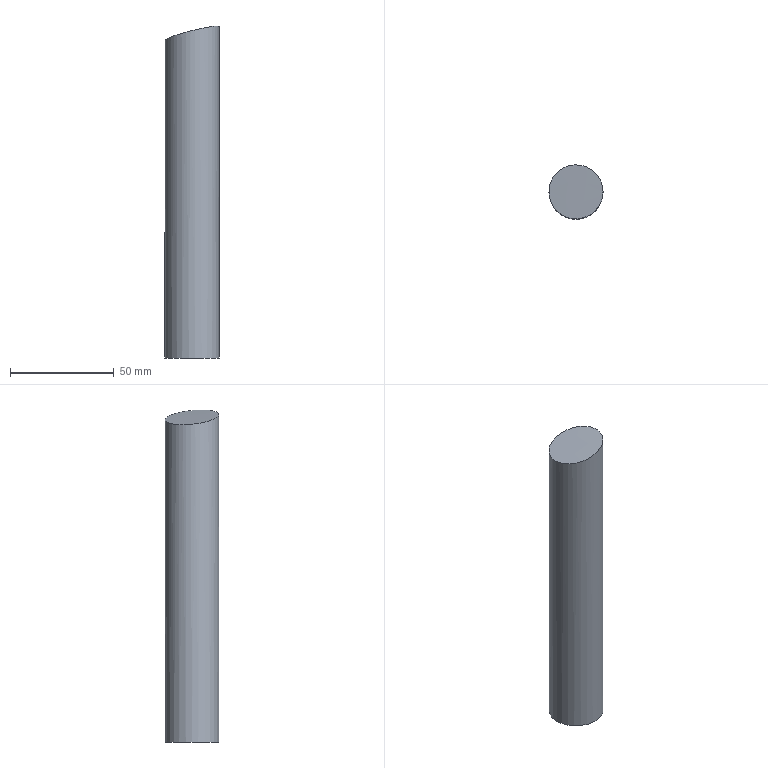Part | NX | features solid 2 | 1 solid | 3 faces | box 26 x 26 x 159.758 mm | volume 82970 mm3 | cylinder 1 | plane 1 | spline 1 | commonest cylinder face diameters 26 x1
STEP:
#1=CARTESIAN_POINT('',(-792.,330.,-138.));
#2=VERTEX_POINT('',#1);
#3=CARTESIAN_POINT('',(-805.,330.,-138.));
#4=DIRECTION('',(0.,0.,-1.));
#5=DIRECTION('',(1.,0.,0.));
#6=AXIS2_PLACEMENT_3D('',#3,#4,#5);
#7=CIRCLE('',#6,13.);
#8=EDGE_CURVE('',#2,#2,#7,.T.);
#9=ORIENTED_EDGE('',*,*,#8,.F.);
#10=EDGE_LOOP('',(#9));
#11=FACE_BOUND('',#10,.T.);
#12=CARTESIAN_POINT('',(-802.129,342.679,17.767));
#13=VERTEX_POINT('',#12);
#14=CARTESIAN_POINT('',(-794.433,338.853,20.068));
#15=CARTESIAN_POINT('',(-801.821,343.999,17.725));
#16=CARTESIAN_POINT('',(-810.751,342.544,15.59));
#17=CARTESIAN_POINT('',(-815.875,337.741,14.744));
#18=CARTESIAN_POINT('',(-818.033,332.897,14.664));
#19=CARTESIAN_POINT('',(-818.129,327.615,15.161));
#20=CARTESIAN_POINT('',(-815.561,321.141,16.463));
#21=CARTESIAN_POINT('',(-808.205,316.014,18.844));
#22=CARTESIAN_POINT('',(-799.271,317.444,20.936));
#23=CARTESIAN_POINT('',(-794.136,322.243,21.743));
#24=CARTESIAN_POINT('',(-791.968,327.089,21.811));
#25=CARTESIAN_POINT('',(-791.871,332.386,21.326));
#26=CARTESIAN_POINT('',(-794.433,338.853,20.068));
#27=CARTESIAN_POINT('',(-801.821,343.999,17.725));
#28=CARTESIAN_POINT('',(-810.751,342.544,15.59));
#29=B_SPLINE_CURVE_WITH_KNOTS('',3,(#14,#15,#16,#17,#18,#19,#20,#21,#22,#23,#24,#25,#26,#27,#28),.UNSPECIFIED.,.T.,.F.,(1,1,1,1,1,1,1,1,1,1,1,1,1,1,1,1,1,1,1),(-0.02068,-0.01551,-0.01034,0.,0.01034,0.01551,0.02068,0.02585,0.03102,0.04136,0.0517,0.05687,0.06204,0.06721,0.07238,0.08272,0.09306,0.09823,0.1034),.UNSPECIFIED.);
#30=EDGE_CURVE('',#13,#13,#29,.T.);
#31=ORIENTED_EDGE('',*,*,#30,.F.);
#32=EDGE_LOOP('',(#31));
#33=FACE_BOUND('',#32,.T.);
#34=CARTESIAN_POINT('',(-805.,330.,-38.));
#35=DIRECTION('',(0.,0.,-1.));
#36=DIRECTION('',(0.,-1.,0.));
#37=AXIS2_PLACEMENT_3D('',#34,#35,#36);
#38=CYLINDRICAL_SURFACE('',#37,13.);
#39=ADVANCED_FACE('',(#11,#33),#38,.T.);
#40=ORIENTED_EDGE('',*,*,#8,.T.);
#41=EDGE_LOOP('',(#40));
#42=FACE_BOUND('',#41,.T.);
#43=CARTESIAN_POINT('',(-805.,330.,-138.));
#44=DIRECTION('',(0.,0.,1.));
#45=DIRECTION('',(0.,1.,0.));
#46=AXIS2_PLACEMENT_3D('',#43,#44,#45);
#47=PLANE('',#46);
#48=ADVANCED_FACE('',(#42),#47,.F.);
#49=ORIENTED_EDGE('',*,*,#30,.T.);
#50=EDGE_LOOP('',(#49));
#51=FACE_BOUND('',#50,.T.);
#52=CARTESIAN_POINT('',(-793.442,315.831,22.5));
#53=CARTESIAN_POINT('',(-802.463,316.506,20.258));
#54=CARTESIAN_POINT('',(-811.291,317.206,17.963));
#55=CARTESIAN_POINT('',(-819.923,317.93,15.616));
#56=CARTESIAN_POINT('',(-792.37,324.635,21.96));
#57=CARTESIAN_POINT('',(-801.367,325.324,19.72));
#58=CARTESIAN_POINT('',(-810.171,326.039,17.428));
#59=CARTESIAN_POINT('',(-818.779,326.779,15.085));
#60=CARTESIAN_POINT('',(-791.248,333.376,21.392));
#61=CARTESIAN_POINT('',(-800.222,334.078,19.156));
#62=CARTESIAN_POINT('',(-809.,334.807,16.867));
#63=CARTESIAN_POINT('',(-817.582,335.561,14.529));
#64=CARTESIAN_POINT('',(-790.079,342.052,20.799));
#65=CARTESIAN_POINT('',(-799.025,342.767,18.566));
#66=CARTESIAN_POINT('',(-807.777,343.509,16.281));
#67=CARTESIAN_POINT('',(-816.332,344.277,13.947));
#68=B_SPLINE_SURFACE_WITH_KNOTS('',3,3,((#52,#53,#54,#55),(#56,#57,#58,#59),(#60,#61,#62,#63),(#64,#65,#66,#67)),.UNSPECIFIED.,.F.,.F.,.F.,(4,4),(4,4),(0.599,0.6506),(0.8968,0.949),.UNSPECIFIED.);
#69=ADVANCED_FACE('',(#51),#68,.T.);
#70=CLOSED_SHELL('',(#39,#48,#69));
#71=MANIFOLD_SOLID_BREP('',#70);
#72=(LENGTH_UNIT()NAMED_UNIT(*)SI_UNIT(.MILLI.,.METRE.));
#73=UNCERTAINTY_MEASURE_WITH_UNIT(LENGTH_MEASURE(0.0508),#72,'','');
#74=(NAMED_UNIT(*)PLANE_ANGLE_UNIT()SI_UNIT($,.RADIAN.));
#75=(NAMED_UNIT(*)SI_UNIT($,.STERADIAN.)SOLID_ANGLE_UNIT());
#76=(GEOMETRIC_REPRESENTATION_CONTEXT(3)GLOBAL_UNCERTAINTY_ASSIGNED_CONTEXT((#73))GLOBAL_UNIT_ASSIGNED_CONTEXT((#72,#74,#75))REPRESENTATION_CONTEXT('',''));
#77=ADVANCED_BREP_SHAPE_REPRESENTATION('',(#71),#76);